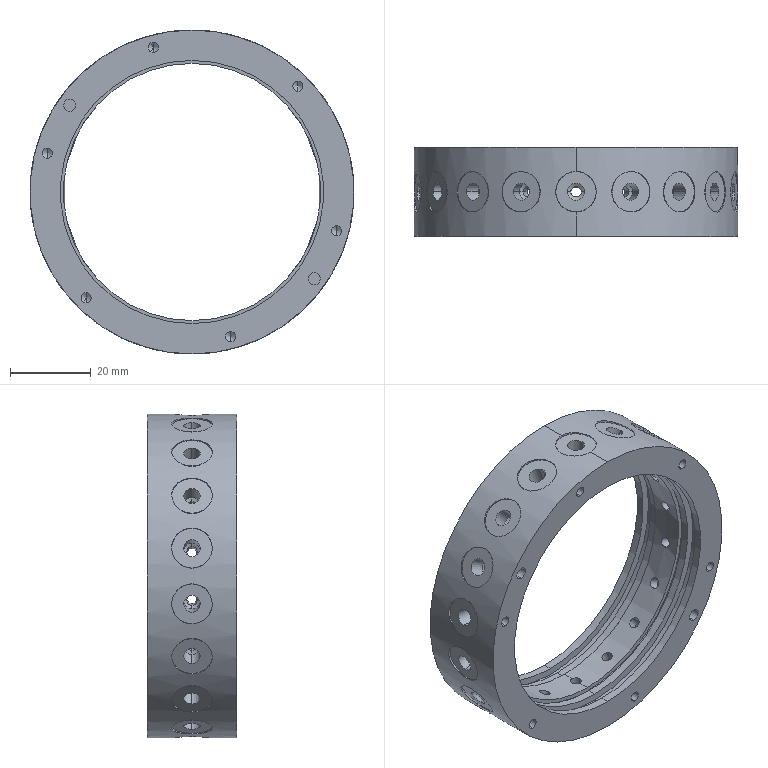Part | SolidWorks | features ICE 6, CirPattern 5, 3DProfileFeature 3, HoleWzd 3, RevCut 2, Cut 1, Extrusion 1, Revolution 1 | 1 solid | 246 faces | box 80 x 22 x 80 mm | volume 34396 mm3 | cylinder 156 | cone 60 | plane 30 | commonest cylinder face diameters 2.6 x36 4.2 x36 10 x36 2.5 x24 65 x8 3 x4